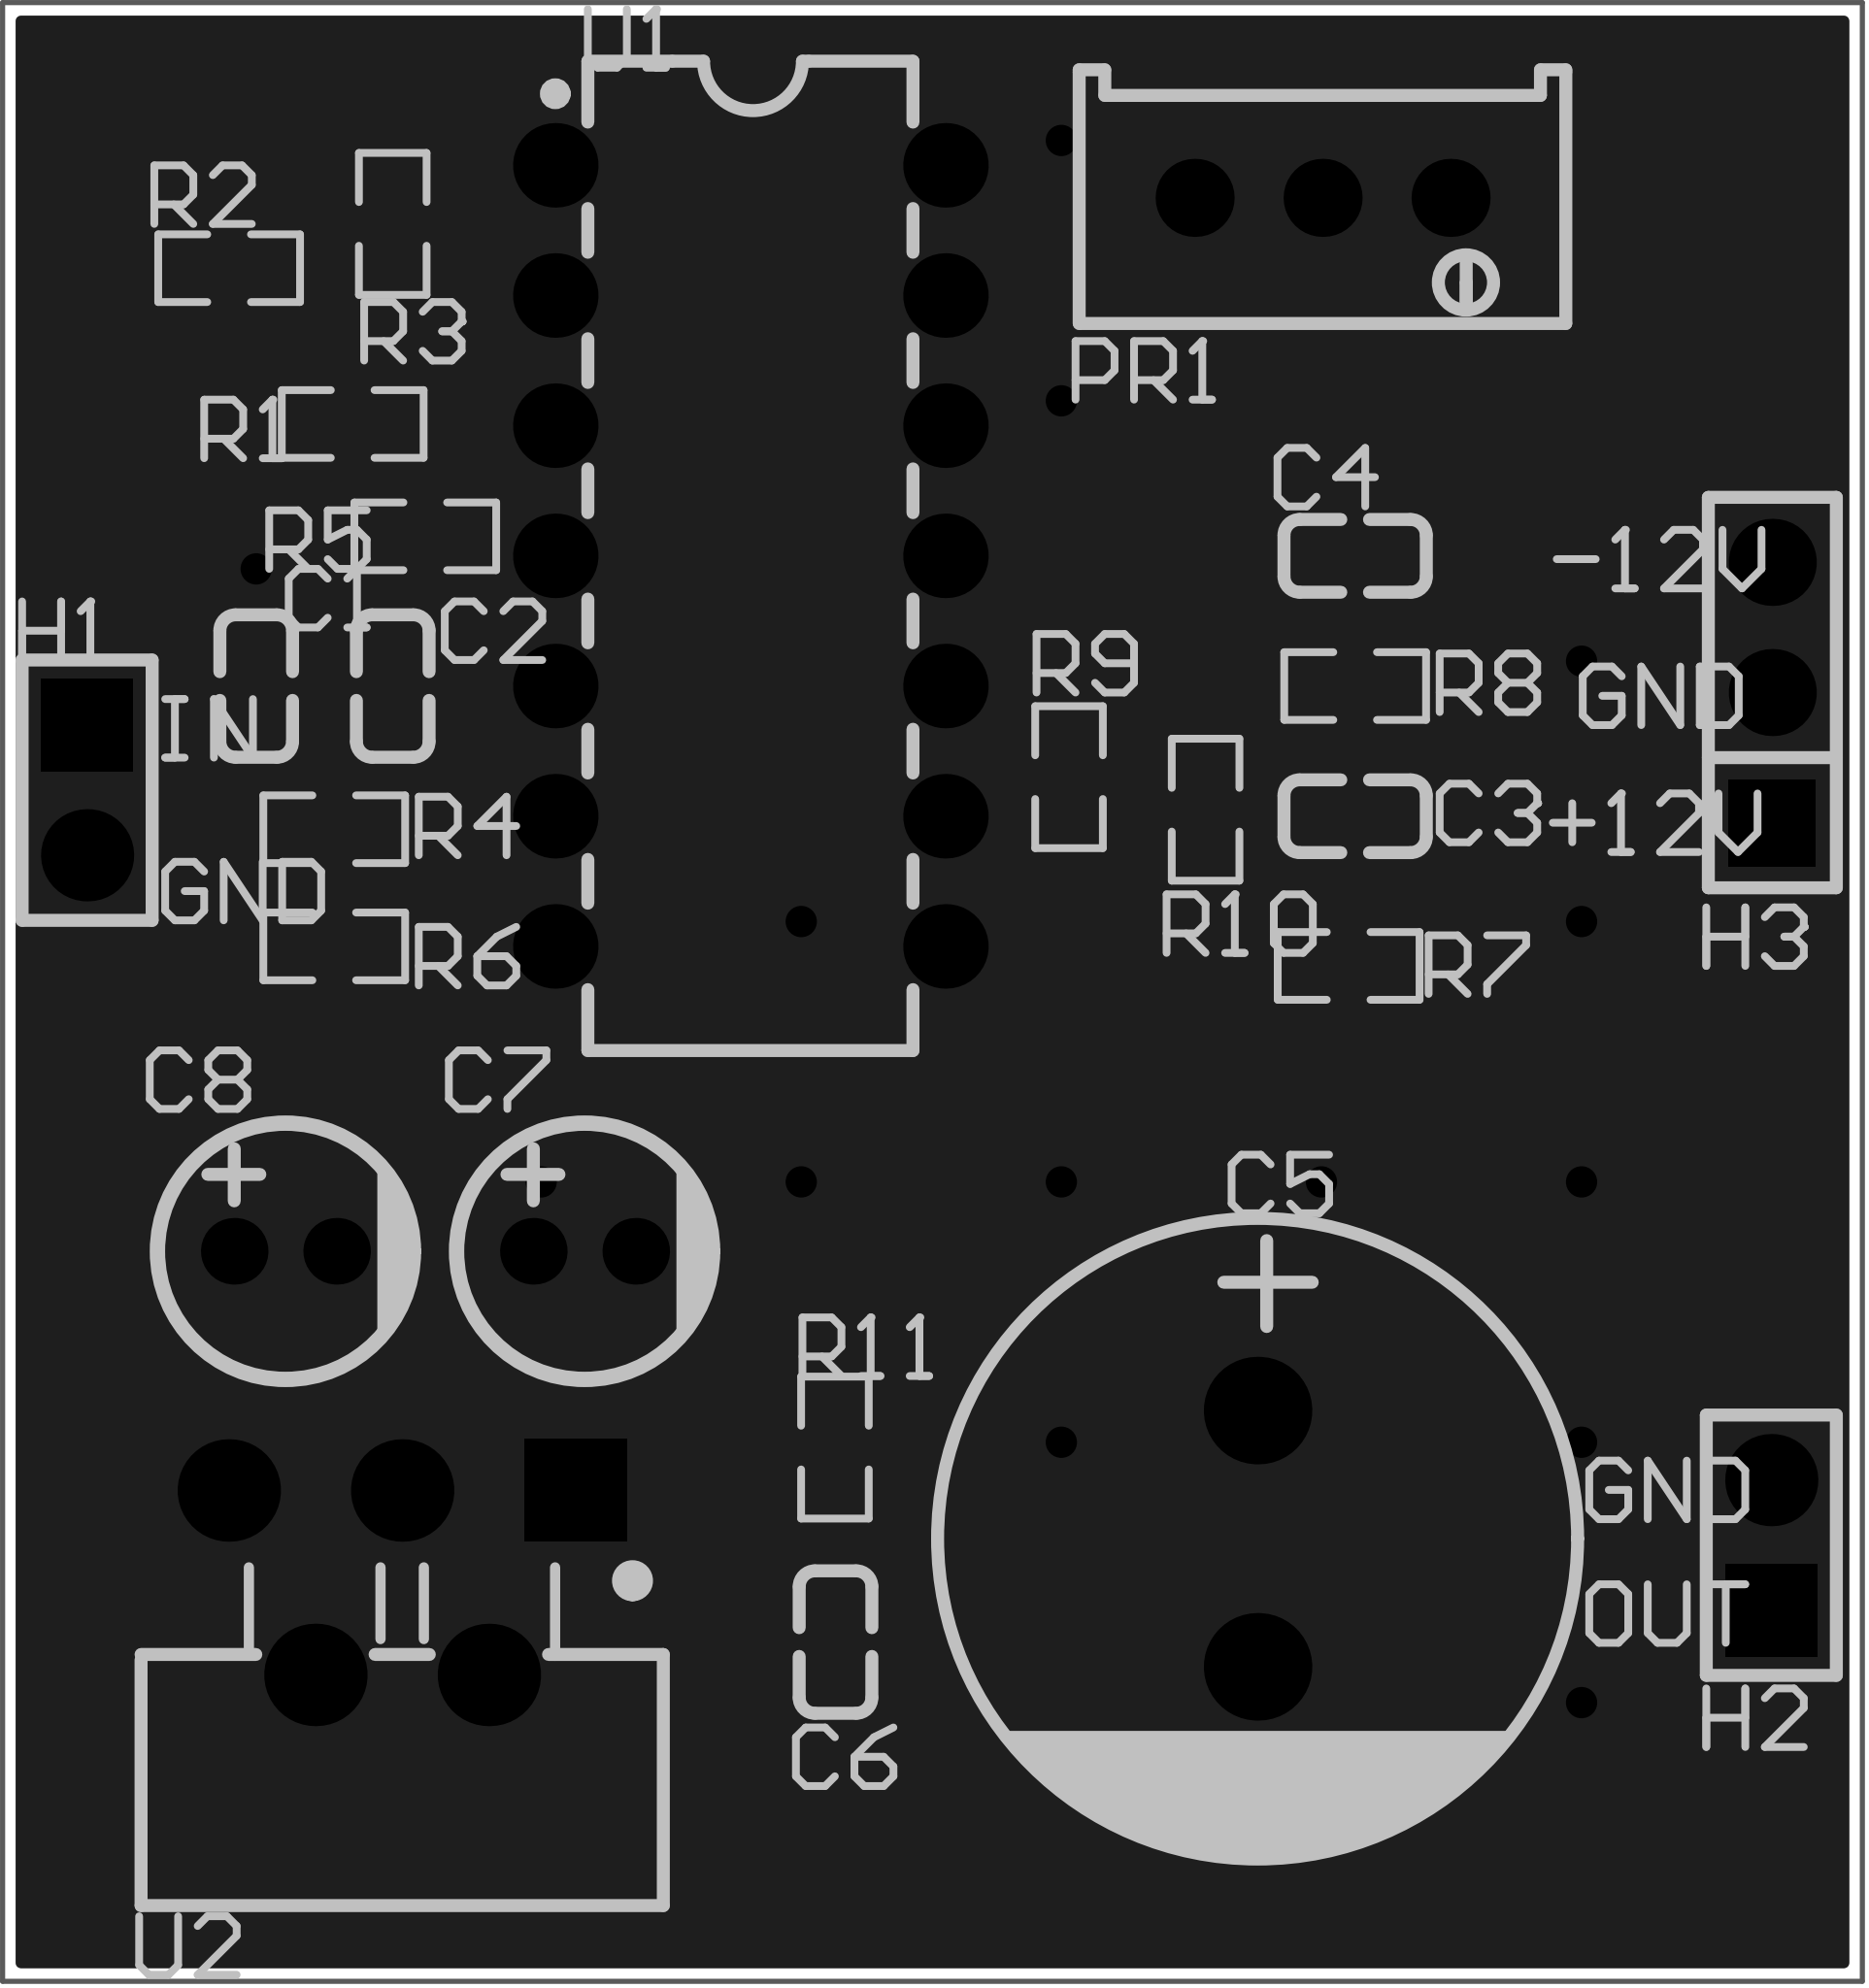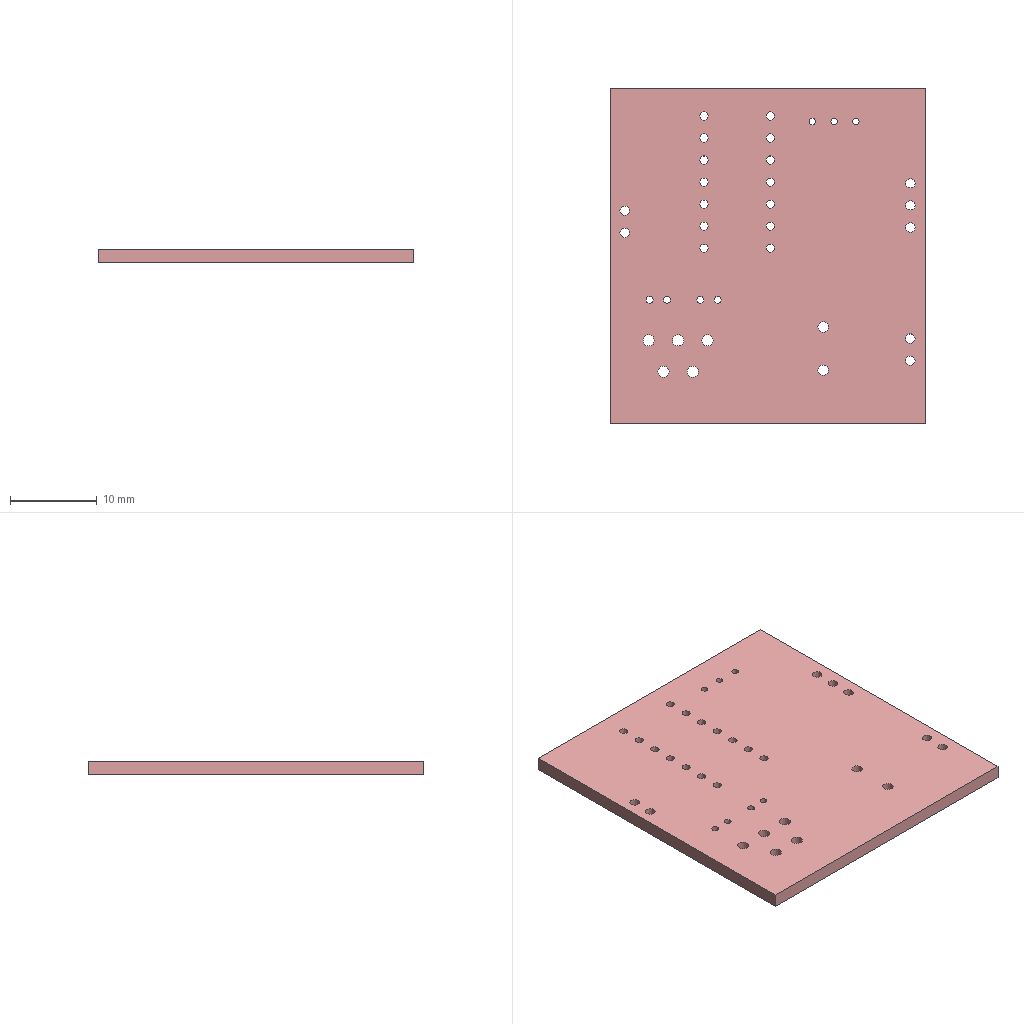Circuit board layout | Altium Designer | box 36.3 x 38.6 x 1.6 mm
Layer stack:
# Altium Designer layer stack of  (unit mm; dielectric type: 0 none, 1 core, 2 prepreg, 3 surface material)
index,name,kind,layer,copper_thickness_mm,dielectric_type,dielectric_thickness_mm,dielectric_material,dielectric_constant
0,Top Paste Mask Layer,other,,,,,,
1,Top Silkscreen Layer,other,,,,,,
2,Top Solder Mask Layer,dielectric,,,3,0.01,,3.3
3,Top Layer,copper,Top Layer,0.035,,,,
4,Dielectric1,dielectric,,,3,1.51,FR4,4.5
5,Bottom Layer,copper,Bottom Layer,0.035,,,,
6,Bottom Solder Mask Layer,dielectric,,,3,0.01,,3.3
7,Bottom Silkscreen Layer,other,,,,,,
8,Bottom Paste Mask Layer,other,,,,,,
# drill layer pairs: low layer,high layer
drill_pair,Top Layer,Bottom Layer
Part placement:
Designator,Comment,Layer,Footprint,Center-X(mm),Center-Y(mm),Rotation
C1,100nF,TopLayer,C0603,85.217,104.648,270
C2,100nF,TopLayer,C0603,87.884,104.648,90
C3,10nF,TopLayer,C0603,106.68,102.108,180
C4,10nF,TopLayer,C0603,106.68,107.188,0
C5,1000uF,TopLayer,CAP-TH_BD12.5-P5.00-D0.6-FD,104.775,88.011,270
C6,0.051UF,TopLayer,C0603,96.532,85.994,270
C7,10uF,TopLayer,CAP-TH_BD5.0-P2.00-D0.8-FD-10UF50VC110GL,91.63,93.619,0
C8,10uF,TopLayer,CAP-TH_BD5.0-P2.00-D0.8-FD-10UF50VC110GL,85.788,93.619,0
H1,,TopLayer,HDR-TH_2P-P2.54-V-M-1,81.915,102.616,270
H2,,TopLayer,HDR-TH_2P-P2.54-V-M-1,114.808,87.884,90
H3,,TopLayer,HDR-TH_3P-P2.54-V-M,114.828,104.521,90
PR1,10kΩ,TopLayer,R_3296,106.045,114.173,180
R1,9.1,TopLayer,R0603,87.101,109.761,0
R2,10K,TopLayer,R0603,84.688,112.801,0
R3,100K,TopLayer,R0603,87.884,113.665,90
R4,15K,TopLayer,R0603,86.741,101.854,0
R5,15K,TopLayer,R0603,88.519,107.569,0
R6,15K,TopLayer,R0603,86.741,99.568,180
R7,15K,TopLayer,R0603,106.553,99.187,0
R8,15K,TopLayer,R0603,106.68,104.648,180
R9,100K,TopLayer,R0603,101.092,102.87,270
R10,27K,TopLayer,R0603,103.759,102.235,270
R11,10,TopLayer,R0603,96.52,89.789,270
U1,LM324N/PB,TopLayer,PDIP-14_L19.2-W6.6-P2.54-LS7.6-BL,94.869,107.188,270
U2,TDA2030A(XBLW),TopLayer,TO-220-5_L10.5-W15.5-P1.70-TL,88.068,87.152,270
Pad and via stacks:
# Altium Designer via and pad stacks of  (unit mm). Each distinct definition once, with the count of objects using it.
# via: kind,start_layer,end_layer,hole_mm,diameter_mm,mode(0 simple;1 top-mid-bottom;2 full stack),diameter_per_layer,count,example_net
# pad: kind,layer,hole_mm,hole_type(0 round;1 square;2 slot),plating,top_size,top_shape(1 round;2 rect;3 octagon;9 rounded rect),mid_size,bottom_size,mode,footprint,size_per_layer,count,example
pad,Top Layer,0,0,plated,0.8x0.9,2,0.8x0.9,0.8x0.9,0,C0603,,10,C1.2
pad,Top Layer,0,0,plated,0.8065x0.864,2,0.8065x0.864,0.8065x0.864,0,R0603,,22,R1.2
pad,Multi-Layer,1.2,0,plated,2.1x2.1,1,2.1x2.1,2.1x2.1,0,CAP-TH_BD12.5-P5.00-D0.6-FD,,2,C5.1
pad,Multi-Layer,0.8,0,plated,1.3x1.3,1,1.3x1.3,1.3x1.3,0,CAP-TH_BD5.0-P2.00-D0.8-FD-10UF50VC110GL,,4,C7.2
pad,Multi-Layer,1.1,0,plated,1.8x1.8,1,1.8x1.8,1.8x1.8,0,HDR-TH_2P-P2.54-V-M-1,,2,H1.2
pad,Multi-Layer,1.1,0,plated,1.8x1.8,2,1.8x1.8,1.8x1.8,0,HDR-TH_2P-P2.54-V-M-1,,2,H1.1
pad,Multi-Layer,1.1,0,plated,1.7x1.7,2,1.7x1.7,1.7x1.7,0,HDR-TH_3P-P2.54-V-M,,1,H3.1
pad,Multi-Layer,1.1,0,plated,1.7x1.7,1,1.7x1.7,1.7x1.7,0,HDR-TH_3P-P2.54-V-M,,2,H3.2
pad,Multi-Layer,0.762,0,plated,1.524x1.524,1,1.524x1.524,1.524x1.524,0,R_3296,,3,PR1.2
pad,Multi-Layer,0.95,0,plated,1.65x1.65,1,1.65x1.65,1.65x1.65,0,PDIP-14_L19.2-W6.6-P2.54-LS7.6-BL,,14,U1.1
pad,Multi-Layer,1.3,0,plated,2x2,2,2x2,2x2,0,TO-220-5_L10.5-W15.5-P1.70-TL,,1,U2.1
pad,Multi-Layer,1.3,0,plated,2x2,1,2x2,2x2,0,TO-220-5_L10.5-W15.5-P1.70-TL,,4,U2.2
via,Top Layer,Bottom Layer,0.3048,0.61,0,,14,$1N10
Copper pours:
name,layer,net,type(0 solid;1 hatched;2 none)
Top Layer-GND,Top Layer,GND,0
Bottom Layer-GND,Bottom Layer,GND,0
Design rules, without the lines most boards share:
# Altium Designer design rules of  (exported by Altium Designer, unit mm)
# columns: name | kind | enabled | priority | scope1 | scope2 | descriptor | typed fields (field=value)
creepage | 65 | enabled | 1 | All | All | Creepage Distance Constraint =(0mil) (All),(All) |